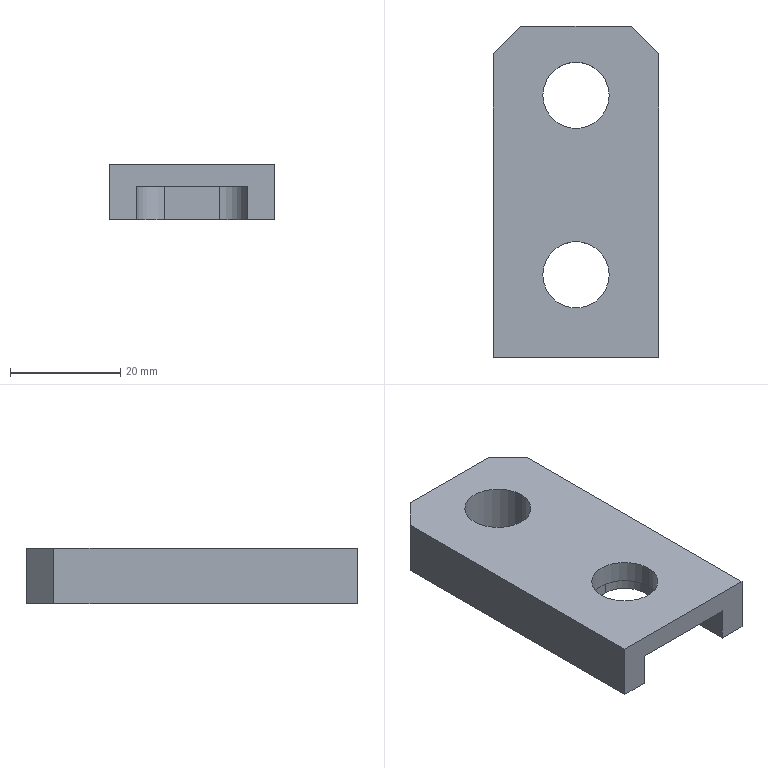Part | STEP file | Polisher connecting part | 1 solid | 18 faces | box 30 x 60 x 10 mm | volume 13231 mm3 | plane 12 | cylinder 6 | commonest cylinder face diameters 12 x4 10 x2
STEP:
#1=CARTESIAN_POINT('',(0.,0.,0.));
#2=DIRECTION('',(0.,0.,1.));
#3=DIRECTION('',(1.,0.,0.));
#4=AXIS2_PLACEMENT_3D('',#1,#2,#3);
#5=CARTESIAN_POINT('',(-6.,47.5,10.));
#6=VERTEX_POINT('',#5);
#7=CARTESIAN_POINT('',(-6.,47.5,0.));
#8=VERTEX_POINT('',#7);
#9=CARTESIAN_POINT('',(-6.,47.5,0.));
#10=DIRECTION('',(0.,0.,-1.));
#11=VECTOR('',#10,1.);
#12=LINE('',#9,#11);
#13=CARTESIAN_POINT('',(0.,47.5,0.));
#14=DIRECTION('',(0.,0.,-1.));
#15=DIRECTION('',(-1.,0.,0.));
#16=AXIS2_PLACEMENT_3D('',#13,#14,#15);
#17=CYLINDRICAL_SURFACE('',#16,6.);
#18=CARTESIAN_POINT('',(6.283,0.));
#19=DIRECTION('',(0.,1.));
#20=VECTOR('',#19,1.);
#21=LINE('',#18,#20);
#22=(GEOMETRIC_REPRESENTATION_CONTEXT(2)PARAMETRIC_REPRESENTATION_CONTEXT()REPRESENTATION_CONTEXT('',''));
#23=DEFINITIONAL_REPRESENTATION('',(#21),#22);
#24=PCURVE('',#17,#23);
#25=CARTESIAN_POINT('',(0.,47.5,0.));
#26=DIRECTION('',(0.,0.,-1.));
#27=DIRECTION('',(-1.,0.,0.));
#28=AXIS2_PLACEMENT_3D('',#25,#26,#27);
#29=CYLINDRICAL_SURFACE('',#28,6.);
#30=CARTESIAN_POINT('',(0.,0.));
#31=DIRECTION('',(0.,1.));
#32=VECTOR('',#31,1.);
#33=LINE('',#30,#32);
#34=(GEOMETRIC_REPRESENTATION_CONTEXT(2)PARAMETRIC_REPRESENTATION_CONTEXT()REPRESENTATION_CONTEXT('',''));
#35=DEFINITIONAL_REPRESENTATION('',(#33),#34);
#36=PCURVE('',#29,#35);
#37=SURFACE_CURVE('',#12,(#24,#36),.PCURVE_S1.);
#38=EDGE_CURVE('',#6,#8,#37,.T.);
#39=ORIENTED_EDGE('',*,*,#38,.T.);
#40=CARTESIAN_POINT('',(6.,47.5,0.));
#41=VERTEX_POINT('',#40);
#42=CARTESIAN_POINT('',(0.,47.5,0.));
#43=DIRECTION('',(0.,0.,-1.));
#44=DIRECTION('',(-1.,0.,0.));
#45=AXIS2_PLACEMENT_3D('',#42,#43,#44);
#46=CIRCLE('',#45,6.);
#47=CARTESIAN_POINT('',(0.,0.));
#48=DIRECTION('',(1.,0.));
#49=VECTOR('',#48,1.);
#50=LINE('',#47,#49);
#51=(GEOMETRIC_REPRESENTATION_CONTEXT(2)PARAMETRIC_REPRESENTATION_CONTEXT()REPRESENTATION_CONTEXT('',''));
#52=DEFINITIONAL_REPRESENTATION('',(#50),#51);
#53=PCURVE('',#17,#52);
#54=CARTESIAN_POINT('',(0.,0.,0.));
#55=DIRECTION('',(0.,0.,1.));
#56=DIRECTION('',(1.,0.,0.));
#57=AXIS2_PLACEMENT_3D('',#54,#55,#56);
#58=PLANE('',#57);
#59=CARTESIAN_POINT('',(-6.,47.5));
#60=CARTESIAN_POINT('',(-6.,57.892));
#61=CARTESIAN_POINT('',(3.,52.696));
#62=CARTESIAN_POINT('',(12.,47.5));
#63=CARTESIAN_POINT('',(3.,42.304));
#64=CARTESIAN_POINT('',(-6.,37.108));
#65=CARTESIAN_POINT('',(-6.,47.5));
#66=(BOUNDED_CURVE()B_SPLINE_CURVE(2,(#59,#60,#61,#62,#63,#64,#65),.UNSPECIFIED.,.T.,.F.)B_SPLINE_CURVE_WITH_KNOTS((1,2,2,2,2,1),(-2.094,0.,2.094,4.189,6.283,8.378),.UNSPECIFIED.)CURVE()GEOMETRIC_REPRESENTATION_ITEM()RATIONAL_B_SPLINE_CURVE((1.,0.5,1.,0.5,1.,0.5,1.))REPRESENTATION_ITEM(''));
#67=(GEOMETRIC_REPRESENTATION_CONTEXT(2)PARAMETRIC_REPRESENTATION_CONTEXT()REPRESENTATION_CONTEXT('',''));
#68=DEFINITIONAL_REPRESENTATION('',(#66),#67);
#69=PCURVE('',#58,#68);
#70=SURFACE_CURVE('',#46,(#53,#69),.PCURVE_S1.);
#71=EDGE_CURVE('',#41,#8,#70,.T.);
#72=ORIENTED_EDGE('',*,*,#71,.F.);
#73=CARTESIAN_POINT('',(6.,47.5,10.));
#74=VERTEX_POINT('',#73);
#75=CARTESIAN_POINT('',(6.,47.5,0.));
#76=DIRECTION('',(0.,0.,-1.));
#77=VECTOR('',#76,1.);
#78=LINE('',#75,#77);
#79=CARTESIAN_POINT('',(3.142,0.));
#80=DIRECTION('',(0.,1.));
#81=VECTOR('',#80,1.);
#82=LINE('',#79,#81);
#83=(GEOMETRIC_REPRESENTATION_CONTEXT(2)PARAMETRIC_REPRESENTATION_CONTEXT()REPRESENTATION_CONTEXT('',''));
#84=DEFINITIONAL_REPRESENTATION('',(#82),#83);
#85=PCURVE('',#17,#84);
#86=CARTESIAN_POINT('',(3.142,0.));
#87=DIRECTION('',(0.,1.));
#88=VECTOR('',#87,1.);
#89=LINE('',#86,#88);
#90=(GEOMETRIC_REPRESENTATION_CONTEXT(2)PARAMETRIC_REPRESENTATION_CONTEXT()REPRESENTATION_CONTEXT('',''));
#91=DEFINITIONAL_REPRESENTATION('',(#89),#90);
#92=PCURVE('',#29,#91);
#93=SURFACE_CURVE('',#78,(#85,#92),.PCURVE_S1.);
#94=EDGE_CURVE('',#74,#41,#93,.T.);
#95=ORIENTED_EDGE('',*,*,#94,.F.);
#96=CARTESIAN_POINT('',(0.,47.5,10.));
#97=DIRECTION('',(0.,0.,-1.));
#98=DIRECTION('',(-1.,0.,0.));
#99=AXIS2_PLACEMENT_3D('',#96,#97,#98);
#100=CIRCLE('',#99,6.);
#101=CARTESIAN_POINT('',(0.,-10.));
#102=DIRECTION('',(1.,0.));
#103=VECTOR('',#102,1.);
#104=LINE('',#101,#103);
#105=(GEOMETRIC_REPRESENTATION_CONTEXT(2)PARAMETRIC_REPRESENTATION_CONTEXT()REPRESENTATION_CONTEXT('',''));
#106=DEFINITIONAL_REPRESENTATION('',(#104),#105);
#107=PCURVE('',#17,#106);
#108=CARTESIAN_POINT('',(0.,0.,10.));
#109=DIRECTION('',(0.,0.,1.));
#110=DIRECTION('',(1.,0.,0.));
#111=AXIS2_PLACEMENT_3D('',#108,#109,#110);
#112=PLANE('',#111);
#113=CARTESIAN_POINT('',(-6.,47.5));
#114=CARTESIAN_POINT('',(-6.,57.892));
#115=CARTESIAN_POINT('',(3.,52.696));
#116=CARTESIAN_POINT('',(12.,47.5));
#117=CARTESIAN_POINT('',(3.,42.304));
#118=CARTESIAN_POINT('',(-6.,37.108));
#119=CARTESIAN_POINT('',(-6.,47.5));
#120=(BOUNDED_CURVE()B_SPLINE_CURVE(2,(#113,#114,#115,#116,#117,#118,#119),.UNSPECIFIED.,.T.,.F.)B_SPLINE_CURVE_WITH_KNOTS((1,2,2,2,2,1),(-2.094,0.,2.094,4.189,6.283,8.378),.UNSPECIFIED.)CURVE()GEOMETRIC_REPRESENTATION_ITEM()RATIONAL_B_SPLINE_CURVE((1.,0.5,1.,0.5,1.,0.5,1.))REPRESENTATION_ITEM(''));
#121=(GEOMETRIC_REPRESENTATION_CONTEXT(2)PARAMETRIC_REPRESENTATION_CONTEXT()REPRESENTATION_CONTEXT('',''));
#122=DEFINITIONAL_REPRESENTATION('',(#120),#121);
#123=PCURVE('',#112,#122);
#124=SURFACE_CURVE('',#100,(#107,#123),.PCURVE_S1.);
#125=EDGE_CURVE('',#74,#6,#124,.T.);
#126=ORIENTED_EDGE('',*,*,#125,.T.);
#127=EDGE_LOOP('',(#39,#72,#95,#126));
#128=FACE_BOUND('',#127,.F.);
#129=ADVANCED_FACE('',(#128),#17,.F.);
#130=CARTESIAN_POINT('',(-6.,15.,10.));
#131=VERTEX_POINT('',#130);
#132=CARTESIAN_POINT('',(-6.,15.,6.));
#133=VERTEX_POINT('',#132);
#134=CARTESIAN_POINT('',(-6.,15.,6.));
#135=DIRECTION('',(0.,0.,-1.));
#136=VECTOR('',#135,1.);
#137=LINE('',#134,#136);
#138=CARTESIAN_POINT('',(0.,15.,6.));
#139=DIRECTION('',(0.,0.,-1.));
#140=DIRECTION('',(-1.,0.,0.));
#141=AXIS2_PLACEMENT_3D('',#138,#139,#140);
#142=CYLINDRICAL_SURFACE('',#141,6.);
#143=CARTESIAN_POINT('',(6.283,0.));
#144=DIRECTION('',(0.,1.));
#145=VECTOR('',#144,1.);
#146=LINE('',#143,#145);
#147=(GEOMETRIC_REPRESENTATION_CONTEXT(2)PARAMETRIC_REPRESENTATION_CONTEXT()REPRESENTATION_CONTEXT('',''));
#148=DEFINITIONAL_REPRESENTATION('',(#146),#147);
#149=PCURVE('',#142,#148);
#150=CARTESIAN_POINT('',(0.,15.,6.));
#151=DIRECTION('',(0.,0.,-1.));
#152=DIRECTION('',(-1.,0.,0.));
#153=AXIS2_PLACEMENT_3D('',#150,#151,#152);
#154=CYLINDRICAL_SURFACE('',#153,6.);
#155=CARTESIAN_POINT('',(0.,0.));
#156=DIRECTION('',(0.,1.));
#157=VECTOR('',#156,1.);
#158=LINE('',#155,#157);
#159=(GEOMETRIC_REPRESENTATION_CONTEXT(2)PARAMETRIC_REPRESENTATION_CONTEXT()REPRESENTATION_CONTEXT('',''));
#160=DEFINITIONAL_REPRESENTATION('',(#158),#159);
#161=PCURVE('',#154,#160);
#162=SURFACE_CURVE('',#137,(#149,#161),.PCURVE_S1.);
#163=EDGE_CURVE('',#131,#133,#162,.T.);
#164=ORIENTED_EDGE('',*,*,#163,.T.);
#165=CARTESIAN_POINT('',(6.,15.,6.));
#166=VERTEX_POINT('',#165);
#167=CARTESIAN_POINT('',(0.,15.,6.));
#168=DIRECTION('',(0.,0.,-1.));
#169=DIRECTION('',(-1.,0.,0.));
#170=AXIS2_PLACEMENT_3D('',#167,#168,#169);
#171=CIRCLE('',#170,6.);
#172=CARTESIAN_POINT('',(0.,0.));
#173=DIRECTION('',(1.,0.));
#174=VECTOR('',#173,1.);
#175=LINE('',#172,#174);
#176=(GEOMETRIC_REPRESENTATION_CONTEXT(2)PARAMETRIC_REPRESENTATION_CONTEXT()REPRESENTATION_CONTEXT('',''));
#177=DEFINITIONAL_REPRESENTATION('',(#175),#176);
#178=PCURVE('',#142,#177);
#179=CARTESIAN_POINT('',(0.,0.,6.));
#180=DIRECTION('',(0.,0.,1.));
#181=DIRECTION('',(1.,0.,0.));
#182=AXIS2_PLACEMENT_3D('',#179,#180,#181);
#183=PLANE('',#182);
#184=CARTESIAN_POINT('',(-6.,15.));
#185=CARTESIAN_POINT('',(-6.,25.392));
#186=CARTESIAN_POINT('',(3.,20.196));
#187=CARTESIAN_POINT('',(12.,15.));
#188=CARTESIAN_POINT('',(3.,9.804));
#189=CARTESIAN_POINT('',(-6.,4.608));
#190=CARTESIAN_POINT('',(-6.,15.));
#191=(BOUNDED_CURVE()B_SPLINE_CURVE(2,(#184,#185,#186,#187,#188,#189,#190),.UNSPECIFIED.,.T.,.F.)B_SPLINE_CURVE_WITH_KNOTS((1,2,2,2,2,1),(-2.094,0.,2.094,4.189,6.283,8.378),.UNSPECIFIED.)CURVE()GEOMETRIC_REPRESENTATION_ITEM()RATIONAL_B_SPLINE_CURVE((1.,0.5,1.,0.5,1.,0.5,1.))REPRESENTATION_ITEM(''));
#192=(GEOMETRIC_REPRESENTATION_CONTEXT(2)PARAMETRIC_REPRESENTATION_CONTEXT()REPRESENTATION_CONTEXT('',''));
#193=DEFINITIONAL_REPRESENTATION('',(#191),#192);
#194=PCURVE('',#183,#193);
#195=SURFACE_CURVE('',#171,(#178,#194),.PCURVE_S1.);
#196=EDGE_CURVE('',#166,#133,#195,.T.);
#197=ORIENTED_EDGE('',*,*,#196,.F.);
#198=CARTESIAN_POINT('',(6.,15.,10.));
#199=VERTEX_POINT('',#198);
#200=CARTESIAN_POINT('',(6.,15.,6.));
#201=DIRECTION('',(0.,0.,-1.));
#202=VECTOR('',#201,1.);
#203=LINE('',#200,#202);
#204=CARTESIAN_POINT('',(3.142,0.));
#205=DIRECTION('',(0.,1.));
#206=VECTOR('',#205,1.);
#207=LINE('',#204,#206);
#208=(GEOMETRIC_REPRESENTATION_CONTEXT(2)PARAMETRIC_REPRESENTATION_CONTEXT()REPRESENTATION_CONTEXT('',''));
#209=DEFINITIONAL_REPRESENTATION('',(#207),#208);
#210=PCURVE('',#142,#209);
#211=CARTESIAN_POINT('',(3.142,0.));
#212=DIRECTION('',(0.,1.));
#213=VECTOR('',#212,1.);
#214=LINE('',#211,#213);
#215=(GEOMETRIC_REPRESENTATION_CONTEXT(2)PARAMETRIC_REPRESENTATION_CONTEXT()REPRESENTATION_CONTEXT('',''));
#216=DEFINITIONAL_REPRESENTATION('',(#214),#215);
#217=PCURVE('',#154,#216);
#218=SURFACE_CURVE('',#203,(#210,#217),.PCURVE_S1.);
#219=EDGE_CURVE('',#199,#166,#218,.T.);
#220=ORIENTED_EDGE('',*,*,#219,.F.);
#221=CARTESIAN_POINT('',(0.,15.,10.));
#222=DIRECTION('',(0.,0.,1.));
#223=DIRECTION('',(1.,0.,0.));
#224=AXIS2_PLACEMENT_3D('',#221,#222,#223);
#225=CIRCLE('',#224,6.);
#226=CARTESIAN_POINT('',(9.425,-4.));
#227=DIRECTION('',(-1.,0.));
#228=VECTOR('',#227,1.);
#229=LINE('',#226,#228);
#230=(GEOMETRIC_REPRESENTATION_CONTEXT(2)PARAMETRIC_REPRESENTATION_CONTEXT()REPRESENTATION_CONTEXT('',''));
#231=DEFINITIONAL_REPRESENTATION('',(#229),#230);
#232=PCURVE('',#142,#231);
#233=CARTESIAN_POINT('',(0.,15.));
#234=DIRECTION('',(1.,0.));
#235=AXIS2_PLACEMENT_2D('',#233,#234);
#236=CIRCLE('',#235,6.);
#237=(GEOMETRIC_REPRESENTATION_CONTEXT(2)PARAMETRIC_REPRESENTATION_CONTEXT()REPRESENTATION_CONTEXT('',''));
#238=DEFINITIONAL_REPRESENTATION('',(#236),#237);
#239=PCURVE('',#112,#238);
#240=SURFACE_CURVE('',#225,(#232,#239),.PCURVE_S1.);
#241=EDGE_CURVE('',#131,#199,#240,.T.);
#242=ORIENTED_EDGE('',*,*,#241,.F.);
#243=EDGE_LOOP('',(#164,#197,#220,#242));
#244=FACE_BOUND('',#243,.F.);
#245=ADVANCED_FACE('',(#244),#142,.F.);
#246=CARTESIAN_POINT('',(0.,47.5,0.));
#247=DIRECTION('',(0.,0.,-1.));
#248=DIRECTION('',(-1.,0.,0.));
#249=AXIS2_PLACEMENT_3D('',#246,#247,#248);
#250=CIRCLE('',#249,6.);
#251=CARTESIAN_POINT('',(-6.,47.5));
#252=CARTESIAN_POINT('',(-6.,57.892));
#253=CARTESIAN_POINT('',(3.,52.696));
#254=CARTESIAN_POINT('',(12.,47.5));
#255=CARTESIAN_POINT('',(3.,42.304));
#256=CARTESIAN_POINT('',(-6.,37.108));
#257=CARTESIAN_POINT('',(-6.,47.5));
#258=(BOUNDED_CURVE()B_SPLINE_CURVE(2,(#251,#252,#253,#254,#255,#256,#257),.UNSPECIFIED.,.T.,.F.)B_SPLINE_CURVE_WITH_KNOTS((1,2,2,2,2,1),(-2.094,0.,2.094,4.189,6.283,8.378),.UNSPECIFIED.)CURVE()GEOMETRIC_REPRESENTATION_ITEM()RATIONAL_B_SPLINE_CURVE((1.,0.5,1.,0.5,1.,0.5,1.))REPRESENTATION_ITEM(''));
#259=(GEOMETRIC_REPRESENTATION_CONTEXT(2)PARAMETRIC_REPRESENTATION_CONTEXT()REPRESENTATION_CONTEXT('',''));
#260=DEFINITIONAL_REPRESENTATION('',(#258),#259);
#261=PCURVE('',#58,#260);
#262=CARTESIAN_POINT('',(0.,0.));
#263=DIRECTION('',(1.,0.));
#264=VECTOR('',#263,1.);
#265=LINE('',#262,#264);
#266=(GEOMETRIC_REPRESENTATION_CONTEXT(2)PARAMETRIC_REPRESENTATION_CONTEXT()REPRESENTATION_CONTEXT('',''));
#267=DEFINITIONAL_REPRESENTATION('',(#265),#266);
#268=PCURVE('',#29,#267);
#269=SURFACE_CURVE('',#250,(#261,#268),.PCURVE_S1.);
#270=EDGE_CURVE('',#8,#41,#269,.T.);
#271=ORIENTED_EDGE('',*,*,#270,.F.);
#272=ORIENTED_EDGE('',*,*,#71,.F.);
#273=EDGE_LOOP('',(#271,#272));
#274=FACE_BOUND('',#273,.T.);
#275=CARTESIAN_POINT('',(10.,60.,0.));
#276=VERTEX_POINT('',#275);
#277=CARTESIAN_POINT('',(-10.,60.,0.));
#278=VERTEX_POINT('',#277);
#279=CARTESIAN_POINT('',(15.,60.,0.));
#280=DIRECTION('',(-1.,0.,0.));
#281=VECTOR('',#280,1.);
#282=LINE('',#279,#281);
#283=CARTESIAN_POINT('',(15.,60.));
#284=DIRECTION('',(-1.,0.));
#285=VECTOR('',#284,1.);
#286=LINE('',#283,#285);
#287=(GEOMETRIC_REPRESENTATION_CONTEXT(2)PARAMETRIC_REPRESENTATION_CONTEXT()REPRESENTATION_CONTEXT('',''));
#288=DEFINITIONAL_REPRESENTATION('',(#286),#287);
#289=PCURVE('',#58,#288);
#290=CARTESIAN_POINT('',(15.,60.,43.541));
#291=DIRECTION('',(0.,-1.,0.));
#292=DIRECTION('',(1.,0.,0.));
#293=AXIS2_PLACEMENT_3D('',#290,#291,#292);
#294=PLANE('',#293);
#295=CARTESIAN_POINT('',(0.,-43.541));
#296=DIRECTION('',(-1.,0.));
#297=VECTOR('',#296,1.);
#298=LINE('',#295,#297);
#299=(GEOMETRIC_REPRESENTATION_CONTEXT(2)PARAMETRIC_REPRESENTATION_CONTEXT()REPRESENTATION_CONTEXT('',''));
#300=DEFINITIONAL_REPRESENTATION('',(#298),#299);
#301=PCURVE('',#294,#300);
#302=SURFACE_CURVE('',#282,(#289,#301),.PCURVE_S1.);
#303=EDGE_CURVE('',#276,#278,#302,.T.);
#304=ORIENTED_EDGE('',*,*,#303,.F.);
#305=CARTESIAN_POINT('',(15.,55.,0.));
#306=VERTEX_POINT('',#305);
#307=CARTESIAN_POINT('',(10.,60.,0.));
#308=DIRECTION('',(0.7071,-0.7071,0.));
#309=VECTOR('',#308,1.);
#310=LINE('',#307,#309);
#311=CARTESIAN_POINT('',(10.,60.));
#312=DIRECTION('',(0.7071,-0.7071));
#313=VECTOR('',#312,1.);
#314=LINE('',#311,#313);
#315=(GEOMETRIC_REPRESENTATION_CONTEXT(2)PARAMETRIC_REPRESENTATION_CONTEXT()REPRESENTATION_CONTEXT('',''));
#316=DEFINITIONAL_REPRESENTATION('',(#314),#315);
#317=PCURVE('',#58,#316);
#318=CARTESIAN_POINT('',(10.,60.,43.541));
#319=DIRECTION('',(-0.7071,-0.7071,0.));
#320=DIRECTION('',(0.,0.,-1.));
#321=AXIS2_PLACEMENT_3D('',#318,#319,#320);
#322=PLANE('',#321);
#323=CARTESIAN_POINT('',(43.541,0.));
#324=DIRECTION('',(0.,1.));
#325=VECTOR('',#324,1.);
#326=LINE('',#323,#325);
#327=(GEOMETRIC_REPRESENTATION_CONTEXT(2)PARAMETRIC_REPRESENTATION_CONTEXT()REPRESENTATION_CONTEXT('',''));
#328=DEFINITIONAL_REPRESENTATION('',(#326),#327);
#329=PCURVE('',#322,#328);
#330=SURFACE_CURVE('',#310,(#317,#329),.PCURVE_S1.);
#331=EDGE_CURVE('',#276,#306,#330,.T.);
#332=ORIENTED_EDGE('',*,*,#331,.T.);
#333=CARTESIAN_POINT('',(15.,0.,0.));
#334=VERTEX_POINT('',#333);
#335=CARTESIAN_POINT('',(15.,0.,0.));
#336=DIRECTION('',(0.,1.,0.));
#337=VECTOR('',#336,1.);
#338=LINE('',#335,#337);
#339=CARTESIAN_POINT('',(15.,0.));
#340=DIRECTION('',(0.,1.));
#341=VECTOR('',#340,1.);
#342=LINE('',#339,#341);
#343=(GEOMETRIC_REPRESENTATION_CONTEXT(2)PARAMETRIC_REPRESENTATION_CONTEXT()REPRESENTATION_CONTEXT('',''));
#344=DEFINITIONAL_REPRESENTATION('',(#342),#343);
#345=PCURVE('',#58,#344);
#346=CARTESIAN_POINT('',(15.,0.,10.));
#347=DIRECTION('',(-1.,0.,0.));
#348=DIRECTION('',(0.,0.,1.));
#349=AXIS2_PLACEMENT_3D('',#346,#347,#348);
#350=PLANE('',#349);
#351=CARTESIAN_POINT('',(-10.,0.));
#352=DIRECTION('',(0.,1.));
#353=VECTOR('',#352,1.);
#354=LINE('',#351,#353);
#355=(GEOMETRIC_REPRESENTATION_CONTEXT(2)PARAMETRIC_REPRESENTATION_CONTEXT()REPRESENTATION_CONTEXT('',''));
#356=DEFINITIONAL_REPRESENTATION('',(#354),#355);
#357=PCURVE('',#350,#356);
#358=SURFACE_CURVE('',#338,(#345,#357),.PCURVE_S1.);
#359=EDGE_CURVE('',#334,#306,#358,.T.);
#360=ORIENTED_EDGE('',*,*,#359,.F.);
#361=CARTESIAN_POINT('',(10.,0.,0.));
#362=VERTEX_POINT('',#361);
#363=CARTESIAN_POINT('',(0.,0.,0.));
#364=DIRECTION('',(-1.,0.,0.));
#365=VECTOR('',#364,1.);
#366=LINE('',#363,#365);
#367=CARTESIAN_POINT('',(0.,0.));
#368=DIRECTION('',(-1.,0.));
#369=VECTOR('',#368,1.);
#370=LINE('',#367,#369);
#371=(GEOMETRIC_REPRESENTATION_CONTEXT(2)PARAMETRIC_REPRESENTATION_CONTEXT()REPRESENTATION_CONTEXT('',''));
#372=DEFINITIONAL_REPRESENTATION('',(#370),#371);
#373=PCURVE('',#58,#372);
#374=CARTESIAN_POINT('',(15.,0.,10.));
#375=DIRECTION('',(0.,1.,0.));
#376=DIRECTION('',(0.,0.,1.));
#377=AXIS2_PLACEMENT_3D('',#374,#375,#376);
#378=PLANE('',#377);
#379=CARTESIAN_POINT('',(-10.,-15.));
#380=DIRECTION('',(0.,-1.));
#381=VECTOR('',#380,1.);
#382=LINE('',#379,#381);
#383=(GEOMETRIC_REPRESENTATION_CONTEXT(2)PARAMETRIC_REPRESENTATION_CONTEXT()REPRESENTATION_CONTEXT('',''));
#384=DEFINITIONAL_REPRESENTATION('',(#382),#383);
#385=PCURVE('',#378,#384);
#386=SURFACE_CURVE('',#366,(#373,#385),.PCURVE_S1.);
#387=EDGE_CURVE('',#334,#362,#386,.T.);
#388=ORIENTED_EDGE('',*,*,#387,.T.);
#389=CARTESIAN_POINT('',(10.,20.,0.));
#390=VERTEX_POINT('',#389);
#391=CARTESIAN_POINT('',(10.,-25.,0.));
#392=DIRECTION('',(0.,1.,0.));
#393=VECTOR('',#392,1.);
#394=LINE('',#391,#393);
#395=CARTESIAN_POINT('',(10.,-25.));
#396=DIRECTION('',(0.,1.));
#397=VECTOR('',#396,1.);
#398=LINE('',#395,#397);
#399=(GEOMETRIC_REPRESENTATION_CONTEXT(2)PARAMETRIC_REPRESENTATION_CONTEXT()REPRESENTATION_CONTEXT('',''));
#400=DEFINITIONAL_REPRESENTATION('',(#398),#399);
#401=PCURVE('',#58,#400);
#402=CARTESIAN_POINT('',(10.,-25.,6.));
#403=DIRECTION('',(-1.,0.,0.));
#404=DIRECTION('',(0.,0.,1.));
#405=AXIS2_PLACEMENT_3D('',#402,#403,#404);
#406=PLANE('',#405);
#407=CARTESIAN_POINT('',(-6.,0.));
#408=DIRECTION('',(0.,1.));
#409=VECTOR('',#408,1.);
#410=LINE('',#407,#409);
#411=(GEOMETRIC_REPRESENTATION_CONTEXT(2)PARAMETRIC_REPRESENTATION_CONTEXT()REPRESENTATION_CONTEXT('',''));
#412=DEFINITIONAL_REPRESENTATION('',(#410),#411);
#413=PCURVE('',#406,#412);
#414=SURFACE_CURVE('',#394,(#401,#413),.PCURVE_S1.);
#415=EDGE_CURVE('',#362,#390,#414,.T.);
#416=ORIENTED_EDGE('',*,*,#415,.T.);
#417=CARTESIAN_POINT('',(5.,25.,0.));
#418=VERTEX_POINT('',#417);
#419=CARTESIAN_POINT('',(5.,20.,0.));
#420=DIRECTION('',(0.,0.,1.));
#421=DIRECTION('',(1.,0.,0.));
#422=AXIS2_PLACEMENT_3D('',#419,#420,#421);
#423=CIRCLE('',#422,5.);
#424=CARTESIAN_POINT('',(5.,20.));
#425=DIRECTION('',(1.,0.));
#426=AXIS2_PLACEMENT_2D('',#424,#425);
#427=CIRCLE('',#426,5.);
#428=(GEOMETRIC_REPRESENTATION_CONTEXT(2)PARAMETRIC_REPRESENTATION_CONTEXT()REPRESENTATION_CONTEXT('',''));
#429=DEFINITIONAL_REPRESENTATION('',(#427),#428);
#430=PCURVE('',#58,#429);
#431=CARTESIAN_POINT('',(5.,20.,6.));
#432=DIRECTION('',(0.,0.,1.));
#433=DIRECTION('',(1.,0.,0.));
#434=AXIS2_PLACEMENT_3D('',#431,#432,#433);
#435=CYLINDRICAL_SURFACE('',#434,5.);
#436=CARTESIAN_POINT('',(0.,-6.));
#437=DIRECTION('',(1.,0.));
#438=VECTOR('',#437,1.);
#439=LINE('',#436,#438);
#440=(GEOMETRIC_REPRESENTATION_CONTEXT(2)PARAMETRIC_REPRESENTATION_CONTEXT()REPRESENTATION_CONTEXT('',''));
#441=DEFINITIONAL_REPRESENTATION('',(#439),#440);
#442=PCURVE('',#435,#441);
#443=SURFACE_CURVE('',#423,(#430,#442),.PCURVE_S1.);
#444=EDGE_CURVE('',#390,#418,#443,.T.);
#445=ORIENTED_EDGE('',*,*,#444,.T.);
#446=CARTESIAN_POINT('',(-5.,25.,0.));
#447=VERTEX_POINT('',#446);
#448=CARTESIAN_POINT('',(10.,25.,0.));
#449=DIRECTION('',(-1.,0.,0.));
#450=VECTOR('',#449,1.);
#451=LINE('',#448,#450);
#452=CARTESIAN_POINT('',(10.,25.));
#453=DIRECTION('',(-1.,0.));
#454=VECTOR('',#453,1.);
#455=LINE('',#452,#454);
#456=(GEOMETRIC_REPRESENTATION_CONTEXT(2)PARAMETRIC_REPRESENTATION_CONTEXT()REPRESENTATION_CONTEXT('',''));
#457=DEFINITIONAL_REPRESENTATION('',(#455),#456);
#458=PCURVE('',#58,#457);
#459=CARTESIAN_POINT('',(10.,25.,6.));
#460=DIRECTION('',(0.,-1.,0.));
#461=DIRECTION('',(0.,0.,-1.));
#462=AXIS2_PLACEMENT_3D('',#459,#460,#461);
#463=PLANE('',#462);
#464=CARTESIAN_POINT('',(6.,0.));
#465=DIRECTION('',(0.,-1.));
#466=VECTOR('',#465,1.);
#467=LINE('',#464,#466);
#468=(GEOMETRIC_REPRESENTATION_CONTEXT(2)PARAMETRIC_REPRESENTATION_CONTEXT()REPRESENTATION_CONTEXT('',''));
#469=DEFINITIONAL_REPRESENTATION('',(#467),#468);
#470=PCURVE('',#463,#469);
#471=SURFACE_CURVE('',#451,(#458,#470),.PCURVE_S1.);
#472=EDGE_CURVE('',#418,#447,#471,.T.);
#473=ORIENTED_EDGE('',*,*,#472,.T.);
#474=CARTESIAN_POINT('',(-10.,20.,0.));
#475=VERTEX_POINT('',#474);
#476=CARTESIAN_POINT('',(-5.,20.,0.));
#477=DIRECTION('',(0.,0.,1.));
#478=DIRECTION('',(1.,0.,0.));
#479=AXIS2_PLACEMENT_3D('',#476,#477,#478);
#480=CIRCLE('',#479,5.);
#481=CARTESIAN_POINT('',(-5.,20.));
#482=DIRECTION('',(1.,0.));
#483=AXIS2_PLACEMENT_2D('',#481,#482);
#484=CIRCLE('',#483,5.);
#485=(GEOMETRIC_REPRESENTATION_CONTEXT(2)PARAMETRIC_REPRESENTATION_CONTEXT()REPRESENTATION_CONTEXT('',''));
#486=DEFINITIONAL_REPRESENTATION('',(#484),#485);
#487=PCURVE('',#58,#486);
#488=CARTESIAN_POINT('',(-5.,20.,6.));
#489=DIRECTION('',(0.,0.,1.));
#490=DIRECTION('',(1.,0.,0.));
#491=AXIS2_PLACEMENT_3D('',#488,#489,#490);
#492=CYLINDRICAL_SURFACE('',#491,5.);
#493=CARTESIAN_POINT('',(0.,-6.));
#494=DIRECTION('',(1.,0.));
#495=VECTOR('',#494,1.);
#496=LINE('',#493,#495);
#497=(GEOMETRIC_REPRESENTATION_CONTEXT(2)PARAMETRIC_REPRESENTATION_CONTEXT()REPRESENTATION_CONTEXT('',''));
#498=DEFINITIONAL_REPRESENTATION('',(#496),#497);
#499=PCURVE('',#492,#498);
#500=SURFACE_CURVE('',#480,(#487,#499),.PCURVE_S1.);
#501=EDGE_CURVE('',#447,#475,#500,.T.);
#502=ORIENTED_EDGE('',*,*,#501,.T.);
#503=CARTESIAN_POINT('',(-10.,0.,0.));
#504=VERTEX_POINT('',#503);
#505=CARTESIAN_POINT('',(-10.,-25.,0.));
#506=DIRECTION('',(0.,-1.,0.));
#507=VECTOR('',#506,1.);
#508=LINE('',#505,#507);
#509=CARTESIAN_POINT('',(-10.,-25.));
#510=DIRECTION('',(0.,-1.));
#511=VECTOR('',#510,1.);
#512=LINE('',#509,#511);
#513=(GEOMETRIC_REPRESENTATION_CONTEXT(2)PARAMETRIC_REPRESENTATION_CONTEXT()REPRESENTATION_CONTEXT('',''));
#514=DEFINITIONAL_REPRESENTATION('',(#512),#513);
#515=PCURVE('',#58,#514);
#516=CARTESIAN_POINT('',(-10.,-25.,6.));
#517=DIRECTION('',(1.,0.,0.));
#518=DIRECTION('',(0.,0.,-1.));
#519=AXIS2_PLACEMENT_3D('',#516,#517,#518);
#520=PLANE('',#519);
#521=CARTESIAN_POINT('',(6.,0.));
#522=DIRECTION('',(0.,-1.));
#523=VECTOR('',#522,1.);
#524=LINE('',#521,#523);
#525=(GEOMETRIC_REPRESENTATION_CONTEXT(2)PARAMETRIC_REPRESENTATION_CONTEXT()REPRESENTATION_CONTEXT('',''));
#526=DEFINITIONAL_REPRESENTATION('',(#524),#525);
#527=PCURVE('',#520,#526);
#528=SURFACE_CURVE('',#508,(#515,#527),.PCURVE_S1.);
#529=EDGE_CURVE('',#475,#504,#528,.T.);
#530=ORIENTED_EDGE('',*,*,#529,.T.);
#531=CARTESIAN_POINT('',(-15.,0.,0.));
#532=VERTEX_POINT('',#531);
#533=CARTESIAN_POINT('',(0.,0.,0.));
#534=DIRECTION('',(-1.,0.,0.));
#535=VECTOR('',#534,1.);
#536=LINE('',#533,#535);
#537=CARTESIAN_POINT('',(0.,0.));
#538=DIRECTION('',(-1.,0.));
#539=VECTOR('',#538,1.);
#540=LINE('',#537,#539);
#541=(GEOMETRIC_REPRESENTATION_CONTEXT(2)PARAMETRIC_REPRESENTATION_CONTEXT()REPRESENTATION_CONTEXT('',''));
#542=DEFINITIONAL_REPRESENTATION('',(#540),#541);
#543=PCURVE('',#58,#542);
#544=CARTESIAN_POINT('',(-10.,-15.));
#545=DIRECTION('',(0.,-1.));
#546=VECTOR('',#545,1.);
#547=LINE('',#544,#546);
#548=(GEOMETRIC_REPRESENTATION_CONTEXT(2)PARAMETRIC_REPRESENTATION_CONTEXT()REPRESENTATION_CONTEXT('',''));
#549=DEFINITIONAL_REPRESENTATION('',(#547),#548);
#550=PCURVE('',#378,#549);
#551=SURFACE_CURVE('',#536,(#543,#550),.PCURVE_S1.);
#552=EDGE_CURVE('',#504,#532,#551,.T.);
#553=ORIENTED_EDGE('',*,*,#552,.T.);
#554=CARTESIAN_POINT('',(-15.,55.,0.));
#555=VERTEX_POINT('',#554);
#556=CARTESIAN_POINT('',(-15.,0.,0.));
#557=DIRECTION('',(0.,-1.,0.));
#558=VECTOR('',#557,1.);
#559=LINE('',#556,#558);
#560=CARTESIAN_POINT('',(-15.,0.));
#561=DIRECTION('',(0.,-1.));
#562=VECTOR('',#561,1.);
#563=LINE('',#560,#562);
#564=(GEOMETRIC_REPRESENTATION_CONTEXT(2)PARAMETRIC_REPRESENTATION_CONTEXT()REPRESENTATION_CONTEXT('',''));
#565=DEFINITIONAL_REPRESENTATION('',(#563),#564);
#566=PCURVE('',#58,#565);
#567=CARTESIAN_POINT('',(-15.,0.,10.));
#568=DIRECTION('',(1.,0.,0.));
#569=DIRECTION('',(0.,0.,-1.));
#570=AXIS2_PLACEMENT_3D('',#567,#568,#569);
#571=PLANE('',#570);
#572=CARTESIAN_POINT('',(10.,0.));
#573=DIRECTION('',(0.,-1.));
#574=VECTOR('',#573,1.);
#575=LINE('',#572,#574);
#576=(GEOMETRIC_REPRESENTATION_CONTEXT(2)PARAMETRIC_REPRESENTATION_CONTEXT()REPRESENTATION_CONTEXT('',''));
#577=DEFINITIONAL_REPRESENTATION('',(#575),#576);
#578=PCURVE('',#571,#577);
#579=SURFACE_CURVE('',#559,(#566,#578),.PCURVE_S1.);
#580=EDGE_CURVE('',#555,#532,#579,.T.);
#581=ORIENTED_EDGE('',*,*,#580,.F.);
#582=CARTESIAN_POINT('',(-15.,55.,0.));
#583=DIRECTION('',(0.7071,0.7071,0.));
#584=VECTOR('',#583,1.);
#585=LINE('',#582,#584);
#586=CARTESIAN_POINT('',(-15.,55.));
#587=DIRECTION('',(0.7071,0.7071));
#588=VECTOR('',#587,1.);
#589=LINE('',#586,#588);
#590=(GEOMETRIC_REPRESENTATION_CONTEXT(2)PARAMETRIC_REPRESENTATION_CONTEXT()REPRESENTATION_CONTEXT('',''));
#591=DEFINITIONAL_REPRESENTATION('',(#589),#590);
#592=PCURVE('',#58,#591);
#593=CARTESIAN_POINT('',(-15.,55.,10.));
#594=DIRECTION('',(0.7071,-0.7071,0.));
#595=DIRECTION('',(0.,0.,-1.));
#596=AXIS2_PLACEMENT_3D('',#593,#594,#595);
#597=PLANE('',#596);
#598=CARTESIAN_POINT('',(10.,0.));
#599=DIRECTION('',(0.,1.));
#600=VECTOR('',#599,1.);
#601=LINE('',#598,#600);
#602=(GEOMETRIC_REPRESENTATION_CONTEXT(2)PARAMETRIC_REPRESENTATION_CONTEXT()REPRESENTATION_CONTEXT('',''));
#603=DEFINITIONAL_REPRESENTATION('',(#601),#602);
#604=PCURVE('',#597,#603);
#605=SURFACE_CURVE('',#585,(#592,#604),.PCURVE_S1.);
#606=EDGE_CURVE('',#555,#278,#605,.T.);
#607=ORIENTED_EDGE('',*,*,#606,.T.);
#608=EDGE_LOOP('',(#304,#332,#360,#388,#416,#445,#473,#502,#530,#553,#581,#607));
#609=FACE_BOUND('',#608,.T.);
#610=ADVANCED_FACE('',(#274,#609),#58,.F.);
#611=CARTESIAN_POINT('',(-10.,0.,6.));
#612=VERTEX_POINT('',#611);
#613=CARTESIAN_POINT('',(-10.,0.,10.));
#614=DIRECTION('',(0.,0.,-1.));
#615=VECTOR('',#614,1.);
#616=LINE('',#613,#615);
#617=CARTESIAN_POINT('',(0.,-25.));
#618=DIRECTION('',(-1.,0.));
#619=VECTOR('',#618,1.);
#620=LINE('',#617,#619);
#621=(GEOMETRIC_REPRESENTATION_CONTEXT(2)PARAMETRIC_REPRESENTATION_CONTEXT()REPRESENTATION_CONTEXT('',''));
#622=DEFINITIONAL_REPRESENTATION('',(#620),#621);
#623=PCURVE('',#378,#622);
#624=CARTESIAN_POINT('',(-4.,25.));
#625=DIRECTION('',(1.,0.));
#626=VECTOR('',#625,1.);
#627=LINE('',#624,#626);
#628=(GEOMETRIC_REPRESENTATION_CONTEXT(2)PARAMETRIC_REPRESENTATION_CONTEXT()REPRESENTATION_CONTEXT('',''));
#629=DEFINITIONAL_REPRESENTATION('',(#627),#628);
#630=PCURVE('',#520,#629);
#631=SURFACE_CURVE('',#616,(#623,#630),.PCURVE_S1.);
#632=EDGE_CURVE('',#612,#504,#631,.T.);
#633=ORIENTED_EDGE('',*,*,#632,.F.);
#634=CARTESIAN_POINT('',(10.,0.,6.));
#635=VERTEX_POINT('',#634);
#636=CARTESIAN_POINT('',(15.,0.,6.));
#637=DIRECTION('',(1.,0.,0.));
#638=VECTOR('',#637,1.);
#639=LINE('',#636,#638);
#640=CARTESIAN_POINT('',(-4.,0.));
#641=DIRECTION('',(0.,1.));
#642=VECTOR('',#641,1.);
#643=LINE('',#640,#642);
#644=(GEOMETRIC_REPRESENTATION_CONTEXT(2)PARAMETRIC_REPRESENTATION_CONTEXT()REPRESENTATION_CONTEXT('',''));
#645=DEFINITIONAL_REPRESENTATION('',(#643),#644);
#646=PCURVE('',#378,#645);
#647=CARTESIAN_POINT('',(15.,0.));
#648=DIRECTION('',(1.,0.));
#649=VECTOR('',#648,1.);
#650=LINE('',#647,#649);
#651=(GEOMETRIC_REPRESENTATION_CONTEXT(2)PARAMETRIC_REPRESENTATION_CONTEXT()REPRESENTATION_CONTEXT('',''));
#652=DEFINITIONAL_REPRESENTATION('',(#650),#651);
#653=PCURVE('',#183,#652);
#654=SURFACE_CURVE('',#639,(#646,#653),.PCURVE_S1.);
#655=EDGE_CURVE('',#612,#635,#654,.T.);
#656=ORIENTED_EDGE('',*,*,#655,.T.);
#657=CARTESIAN_POINT('',(10.,0.,10.));
#658=DIRECTION('',(0.,0.,1.));
#659=VECTOR('',#658,1.);
#660=LINE('',#657,#659);
#661=CARTESIAN_POINT('',(0.,-5.));
#662=DIRECTION('',(1.,0.));
#663=VECTOR('',#662,1.);
#664=LINE('',#661,#663);
#665=(GEOMETRIC_REPRESENTATION_CONTEXT(2)PARAMETRIC_REPRESENTATION_CONTEXT()REPRESENTATION_CONTEXT('',''));
#666=DEFINITIONAL_REPRESENTATION('',(#664),#665);
#667=PCURVE('',#378,#666);
#668=CARTESIAN_POINT('',(4.,25.));
#669=DIRECTION('',(1.,0.));
#670=VECTOR('',#669,1.);
#671=LINE('',#668,#670);
#672=(GEOMETRIC_REPRESENTATION_CONTEXT(2)PARAMETRIC_REPRESENTATION_CONTEXT()REPRESENTATION_CONTEXT('',''));
#673=DEFINITIONAL_REPRESENTATION('',(#671),#672);
#674=PCURVE('',#406,#673);
#675=SURFACE_CURVE('',#660,(#667,#674),.PCURVE_S1.);
#676=EDGE_CURVE('',#362,#635,#675,.T.);
#677=ORIENTED_EDGE('',*,*,#676,.F.);
#678=ORIENTED_EDGE('',*,*,#387,.F.);
#679=CARTESIAN_POINT('',(15.,0.,10.));
#680=VERTEX_POINT('',#679);
#681=CARTESIAN_POINT('',(15.,0.,10.));
#682=DIRECTION('',(0.,0.,-1.));
#683=VECTOR('',#682,1.);
#684=LINE('',#681,#683);
#685=CARTESIAN_POINT('',(0.,0.));
#686=DIRECTION('',(-1.,0.));
#687=VECTOR('',#686,1.);
#688=LINE('',#685,#687);
#689=(GEOMETRIC_REPRESENTATION_CONTEXT(2)PARAMETRIC_REPRESENTATION_CONTEXT()REPRESENTATION_CONTEXT('',''));
#690=DEFINITIONAL_REPRESENTATION('',(#688),#689);
#691=PCURVE('',#378,#690);
#692=CARTESIAN_POINT('',(0.,0.));
#693=DIRECTION('',(-1.,0.));
#694=VECTOR('',#693,1.);
#695=LINE('',#692,#694);
#696=(GEOMETRIC_REPRESENTATION_CONTEXT(2)PARAMETRIC_REPRESENTATION_CONTEXT()REPRESENTATION_CONTEXT('',''));
#697=DEFINITIONAL_REPRESENTATION('',(#695),#696);
#698=PCURVE('',#350,#697);
#699=SURFACE_CURVE('',#684,(#691,#698),.PCURVE_S1.);
#700=EDGE_CURVE('',#680,#334,#699,.T.);
#701=ORIENTED_EDGE('',*,*,#700,.F.);
#702=CARTESIAN_POINT('',(-15.,0.,10.));
#703=VERTEX_POINT('',#702);
#704=CARTESIAN_POINT('',(15.,0.,10.));
#705=DIRECTION('',(1.,0.,0.));
#706=VECTOR('',#705,1.);
#707=LINE('',#704,#706);
#708=CARTESIAN_POINT('',(0.,0.));
#709=DIRECTION('',(0.,1.));
#710=VECTOR('',#709,1.);
#711=LINE('',#708,#710);
#712=(GEOMETRIC_REPRESENTATION_CONTEXT(2)PARAMETRIC_REPRESENTATION_CONTEXT()REPRESENTATION_CONTEXT('',''));
#713=DEFINITIONAL_REPRESENTATION('',(#711),#712);
#714=PCURVE('',#378,#713);
#715=CARTESIAN_POINT('',(15.,0.));
#716=DIRECTION('',(1.,0.));
#717=VECTOR('',#716,1.);
#718=LINE('',#715,#717);
#719=(GEOMETRIC_REPRESENTATION_CONTEXT(2)PARAMETRIC_REPRESENTATION_CONTEXT()REPRESENTATION_CONTEXT('',''));
#720=DEFINITIONAL_REPRESENTATION('',(#718),#719);
#721=PCURVE('',#112,#720);
#722=SURFACE_CURVE('',#707,(#714,#721),.PCURVE_S1.);
#723=EDGE_CURVE('',#703,#680,#722,.T.);
#724=ORIENTED_EDGE('',*,*,#723,.F.);
#725=CARTESIAN_POINT('',(-15.,0.,10.));
#726=DIRECTION('',(0.,0.,-1.));
#727=VECTOR('',#726,1.);
#728=LINE('',#725,#727);
#729=CARTESIAN_POINT('',(0.,-30.));
#730=DIRECTION('',(-1.,0.));
#731=VECTOR('',#730,1.);
#732=LINE('',#729,#731);
#733=(GEOMETRIC_REPRESENTATION_CONTEXT(2)PARAMETRIC_REPRESENTATION_CONTEXT()REPRESENTATION_CONTEXT('',''));
#734=DEFINITIONAL_REPRESENTATION('',(#732),#733);
#735=PCURVE('',#378,#734);
#736=CARTESIAN_POINT('',(0.,0.));
#737=DIRECTION('',(1.,0.));
#738=VECTOR('',#737,1.);
#739=LINE('',#736,#738);
#740=(GEOMETRIC_REPRESENTATION_CONTEXT(2)PARAMETRIC_REPRESENTATION_CONTEXT()REPRESENTATION_CONTEXT('',''));
#741=DEFINITIONAL_REPRESENTATION('',(#739),#740);
#742=PCURVE('',#571,#741);
#743=SURFACE_CURVE('',#728,(#735,#742),.PCURVE_S1.);
#744=EDGE_CURVE('',#703,#532,#743,.T.);
#745=ORIENTED_EDGE('',*,*,#744,.T.);
#746=ORIENTED_EDGE('',*,*,#552,.F.);
#747=EDGE_LOOP('',(#633,#656,#677,#678,#701,#724,#745,#746));
#748=FACE_BOUND('',#747,.T.);
#749=ADVANCED_FACE('',(#748),#378,.F.);
#750=ORIENTED_EDGE('',*,*,#359,.T.);
#751=CARTESIAN_POINT('',(15.,55.,10.));
#752=VERTEX_POINT('',#751);
#753=CARTESIAN_POINT('',(15.,55.,10.));
#754=DIRECTION('',(0.,0.,1.));
#755=VECTOR('',#754,1.);
#756=LINE('',#753,#755);
#757=CARTESIAN_POINT('',(0.,55.));
#758=DIRECTION('',(1.,0.));
#759=VECTOR('',#758,1.);
#760=LINE('',#757,#759);
#761=(GEOMETRIC_REPRESENTATION_CONTEXT(2)PARAMETRIC_REPRESENTATION_CONTEXT()REPRESENTATION_CONTEXT('',''));
#762=DEFINITIONAL_REPRESENTATION('',(#760),#761);
#763=PCURVE('',#350,#762);
#764=CARTESIAN_POINT('',(33.541,7.071));
#765=DIRECTION('',(-1.,0.));
#766=VECTOR('',#765,1.);
#767=LINE('',#764,#766);
#768=(GEOMETRIC_REPRESENTATION_CONTEXT(2)PARAMETRIC_REPRESENTATION_CONTEXT()REPRESENTATION_CONTEXT('',''));
#769=DEFINITIONAL_REPRESENTATION('',(#767),#768);
#770=PCURVE('',#322,#769);
#771=SURFACE_CURVE('',#756,(#763,#770),.PCURVE_S1.);
#772=EDGE_CURVE('',#306,#752,#771,.T.);
#773=ORIENTED_EDGE('',*,*,#772,.T.);
#774=CARTESIAN_POINT('',(15.,0.,10.));
#775=DIRECTION('',(0.,1.,0.));
#776=VECTOR('',#775,1.);
#777=LINE('',#774,#776);
#778=CARTESIAN_POINT('',(0.,0.));
#779=DIRECTION('',(0.,1.));
#780=VECTOR('',#779,1.);
#781=LINE('',#778,#780);
#782=(GEOMETRIC_REPRESENTATION_CONTEXT(2)PARAMETRIC_REPRESENTATION_CONTEXT()REPRESENTATION_CONTEXT('',''));
#783=DEFINITIONAL_REPRESENTATION('',(#781),#782);
#784=PCURVE('',#350,#783);
#785=CARTESIAN_POINT('',(15.,0.));
#786=DIRECTION('',(0.,1.));
#787=VECTOR('',#786,1.);
#788=LINE('',#785,#787);
#789=(GEOMETRIC_REPRESENTATION_CONTEXT(2)PARAMETRIC_REPRESENTATION_CONTEXT()REPRESENTATION_CONTEXT('',''));
#790=DEFINITIONAL_REPRESENTATION('',(#788),#789);
#791=PCURVE('',#112,#790);
#792=SURFACE_CURVE('',#777,(#784,#791),.PCURVE_S1.);
#793=EDGE_CURVE('',#680,#752,#792,.T.);
#794=ORIENTED_EDGE('',*,*,#793,.F.);
#795=ORIENTED_EDGE('',*,*,#700,.T.);
#796=EDGE_LOOP('',(#750,#773,#794,#795));
#797=FACE_BOUND('',#796,.T.);
#798=ADVANCED_FACE('',(#797),#350,.F.);
#799=CARTESIAN_POINT('',(-15.,55.,10.));
#800=VERTEX_POINT('',#799);
#801=CARTESIAN_POINT('',(-15.,0.,10.));
#802=DIRECTION('',(0.,-1.,0.));
#803=VECTOR('',#802,1.);
#804=LINE('',#801,#803);
#805=CARTESIAN_POINT('',(0.,0.));
#806=DIRECTION('',(0.,-1.));
#807=VECTOR('',#806,1.);
#808=LINE('',#805,#807);
#809=(GEOMETRIC_REPRESENTATION_CONTEXT(2)PARAMETRIC_REPRESENTATION_CONTEXT()REPRESENTATION_CONTEXT('',''));
#810=DEFINITIONAL_REPRESENTATION('',(#808),#809);
#811=PCURVE('',#571,#810);
#812=CARTESIAN_POINT('',(-15.,0.));
#813=DIRECTION('',(0.,-1.));
#814=VECTOR('',#813,1.);
#815=LINE('',#812,#814);
#816=(GEOMETRIC_REPRESENTATION_CONTEXT(2)PARAMETRIC_REPRESENTATION_CONTEXT()REPRESENTATION_CONTEXT('',''));
#817=DEFINITIONAL_REPRESENTATION('',(#815),#816);
#818=PCURVE('',#112,#817);
#819=SURFACE_CURVE('',#804,(#811,#818),.PCURVE_S1.);
#820=EDGE_CURVE('',#800,#703,#819,.T.);
#821=ORIENTED_EDGE('',*,*,#820,.F.);
#822=CARTESIAN_POINT('',(-15.,55.,10.));
#823=DIRECTION('',(0.,0.,-1.));
#824=VECTOR('',#823,1.);
#825=LINE('',#822,#824);
#826=CARTESIAN_POINT('',(0.,55.));
#827=DIRECTION('',(1.,0.));
#828=VECTOR('',#827,1.);
#829=LINE('',#826,#828);
#830=(GEOMETRIC_REPRESENTATION_CONTEXT(2)PARAMETRIC_REPRESENTATION_CONTEXT()REPRESENTATION_CONTEXT('',''));
#831=DEFINITIONAL_REPRESENTATION('',(#829),#830);
#832=PCURVE('',#571,#831);
#833=CARTESIAN_POINT('',(0.,0.));
#834=DIRECTION('',(1.,0.));
#835=VECTOR('',#834,1.);
#836=LINE('',#833,#835);
#837=(GEOMETRIC_REPRESENTATION_CONTEXT(2)PARAMETRIC_REPRESENTATION_CONTEXT()REPRESENTATION_CONTEXT('',''));
#838=DEFINITIONAL_REPRESENTATION('',(#836),#837);
#839=PCURVE('',#597,#838);
#840=SURFACE_CURVE('',#825,(#832,#839),.PCURVE_S1.);
#841=EDGE_CURVE('',#800,#555,#840,.T.);
#842=ORIENTED_EDGE('',*,*,#841,.T.);
#843=ORIENTED_EDGE('',*,*,#580,.T.);
#844=ORIENTED_EDGE('',*,*,#744,.F.);
#845=EDGE_LOOP('',(#821,#842,#843,#844));
#846=FACE_BOUND('',#845,.T.);
#847=ADVANCED_FACE('',(#846),#571,.F.);
#848=CARTESIAN_POINT('',(0.,47.5,10.));
#849=DIRECTION('',(0.,0.,-1.));
#850=DIRECTION('',(-1.,0.,0.));
#851=AXIS2_PLACEMENT_3D('',#848,#849,#850);
#852=CIRCLE('',#851,6.);
#853=CARTESIAN_POINT('',(-6.,47.5));
#854=CARTESIAN_POINT('',(-6.,57.892));
#855=CARTESIAN_POINT('',(3.,52.696));
#856=CARTESIAN_POINT('',(12.,47.5));
#857=CARTESIAN_POINT('',(3.,42.304));
#858=CARTESIAN_POINT('',(-6.,37.108));
#859=CARTESIAN_POINT('',(-6.,47.5));
#860=(BOUNDED_CURVE()B_SPLINE_CURVE(2,(#853,#854,#855,#856,#857,#858,#859),.UNSPECIFIED.,.T.,.F.)B_SPLINE_CURVE_WITH_KNOTS((1,2,2,2,2,1),(-2.094,0.,2.094,4.189,6.283,8.378),.UNSPECIFIED.)CURVE()GEOMETRIC_REPRESENTATION_ITEM()RATIONAL_B_SPLINE_CURVE((1.,0.5,1.,0.5,1.,0.5,1.))REPRESENTATION_ITEM(''));
#861=(GEOMETRIC_REPRESENTATION_CONTEXT(2)PARAMETRIC_REPRESENTATION_CONTEXT()REPRESENTATION_CONTEXT('',''));
#862=DEFINITIONAL_REPRESENTATION('',(#860),#861);
#863=PCURVE('',#112,#862);
#864=CARTESIAN_POINT('',(0.,-10.));
#865=DIRECTION('',(1.,0.));
#866=VECTOR('',#865,1.);
#867=LINE('',#864,#866);
#868=(GEOMETRIC_REPRESENTATION_CONTEXT(2)PARAMETRIC_REPRESENTATION_CONTEXT()REPRESENTATION_CONTEXT('',''));
#869=DEFINITIONAL_REPRESENTATION('',(#867),#868);
#870=PCURVE('',#29,#869);
#871=SURFACE_CURVE('',#852,(#863,#870),.PCURVE_S1.);
#872=EDGE_CURVE('',#6,#74,#871,.T.);
#873=ORIENTED_EDGE('',*,*,#872,.T.);
#874=ORIENTED_EDGE('',*,*,#125,.T.);
#875=EDGE_LOOP('',(#873,#874));
#876=FACE_BOUND('',#875,.T.);
#877=ORIENTED_EDGE('',*,*,#241,.F.);
#878=CARTESIAN_POINT('',(0.,15.,10.));
#879=DIRECTION('',(0.,0.,1.));
#880=DIRECTION('',(1.,0.,0.));
#881=AXIS2_PLACEMENT_3D('',#878,#879,#880);
#882=CIRCLE('',#881,6.);
#883=CARTESIAN_POINT('',(0.,15.));
#884=DIRECTION('',(1.,0.));
#885=AXIS2_PLACEMENT_2D('',#883,#884);
#886=CIRCLE('',#885,6.);
#887=(GEOMETRIC_REPRESENTATION_CONTEXT(2)PARAMETRIC_REPRESENTATION_CONTEXT()REPRESENTATION_CONTEXT('',''));
#888=DEFINITIONAL_REPRESENTATION('',(#886),#887);
#889=PCURVE('',#112,#888);
#890=CARTESIAN_POINT('',(3.142,-4.));
#891=DIRECTION('',(-1.,0.));
#892=VECTOR('',#891,1.);
#893=LINE('',#890,#892);
#894=(GEOMETRIC_REPRESENTATION_CONTEXT(2)PARAMETRIC_REPRESENTATION_CONTEXT()REPRESENTATION_CONTEXT('',''));
#895=DEFINITIONAL_REPRESENTATION('',(#893),#894);
#896=PCURVE('',#154,#895);
#897=SURFACE_CURVE('',#882,(#889,#896),.PCURVE_S1.);
#898=EDGE_CURVE('',#199,#131,#897,.T.);
#899=ORIENTED_EDGE('',*,*,#898,.F.);
#900=EDGE_LOOP('',(#877,#899));
#901=FACE_BOUND('',#900,.T.);
#902=ORIENTED_EDGE('',*,*,#793,.T.);
#903=CARTESIAN_POINT('',(10.,60.,10.));
#904=VERTEX_POINT('',#903);
#905=CARTESIAN_POINT('',(35.,35.,10.));
#906=DIRECTION('',(-0.7071,0.7071,0.));
#907=VECTOR('',#906,1.);
#908=LINE('',#905,#907);
#909=CARTESIAN_POINT('',(35.,35.));
#910=DIRECTION('',(-0.7071,0.7071));
#911=VECTOR('',#910,1.);
#912=LINE('',#909,#911);
#913=(GEOMETRIC_REPRESENTATION_CONTEXT(2)PARAMETRIC_REPRESENTATION_CONTEXT()REPRESENTATION_CONTEXT('',''));
#914=DEFINITIONAL_REPRESENTATION('',(#912),#913);
#915=PCURVE('',#112,#914);
#916=CARTESIAN_POINT('',(33.541,35.355));
#917=DIRECTION('',(0.,-1.));
#918=VECTOR('',#917,1.);
#919=LINE('',#916,#918);
#920=(GEOMETRIC_REPRESENTATION_CONTEXT(2)PARAMETRIC_REPRESENTATION_CONTEXT()REPRESENTATION_CONTEXT('',''));
#921=DEFINITIONAL_REPRESENTATION('',(#919),#920);
#922=PCURVE('',#322,#921);
#923=SURFACE_CURVE('',#908,(#915,#922),.PCURVE_S1.);
#924=EDGE_CURVE('',#752,#904,#923,.T.);
#925=ORIENTED_EDGE('',*,*,#924,.T.);
#926=CARTESIAN_POINT('',(-10.,60.,10.));
#927=VERTEX_POINT('',#926);
#928=CARTESIAN_POINT('',(15.,60.,10.));
#929=DIRECTION('',(-1.,0.,0.));
#930=VECTOR('',#929,1.);
#931=LINE('',#928,#930);
#932=CARTESIAN_POINT('',(15.,60.));
#933=DIRECTION('',(-1.,0.));
#934=VECTOR('',#933,1.);
#935=LINE('',#932,#934);
#936=(GEOMETRIC_REPRESENTATION_CONTEXT(2)PARAMETRIC_REPRESENTATION_CONTEXT()REPRESENTATION_CONTEXT('',''));
#937=DEFINITIONAL_REPRESENTATION('',(#935),#936);
#938=PCURVE('',#112,#937);
#939=CARTESIAN_POINT('',(0.,-33.541));
#940=DIRECTION('',(-1.,0.));
#941=VECTOR('',#940,1.);
#942=LINE('',#939,#941);
#943=(GEOMETRIC_REPRESENTATION_CONTEXT(2)PARAMETRIC_REPRESENTATION_CONTEXT()REPRESENTATION_CONTEXT('',''));
#944=DEFINITIONAL_REPRESENTATION('',(#942),#943);
#945=PCURVE('',#294,#944);
#946=SURFACE_CURVE('',#931,(#938,#945),.PCURVE_S1.);
#947=EDGE_CURVE('',#904,#927,#946,.T.);
#948=ORIENTED_EDGE('',*,*,#947,.T.);
#949=CARTESIAN_POINT('',(-35.,35.,10.));
#950=DIRECTION('',(-0.7071,-0.7071,0.));
#951=VECTOR('',#950,1.);
#952=LINE('',#949,#951);
#953=CARTESIAN_POINT('',(-35.,35.));
#954=DIRECTION('',(-0.7071,-0.7071));
#955=VECTOR('',#954,1.);
#956=LINE('',#953,#955);
#957=(GEOMETRIC_REPRESENTATION_CONTEXT(2)PARAMETRIC_REPRESENTATION_CONTEXT()REPRESENTATION_CONTEXT('',''));
#958=DEFINITIONAL_REPRESENTATION('',(#956),#957);
#959=PCURVE('',#112,#958);
#960=CARTESIAN_POINT('',(0.,-28.284));
#961=DIRECTION('',(0.,-1.));
#962=VECTOR('',#961,1.);
#963=LINE('',#960,#962);
#964=(GEOMETRIC_REPRESENTATION_CONTEXT(2)PARAMETRIC_REPRESENTATION_CONTEXT()REPRESENTATION_CONTEXT('',''));
#965=DEFINITIONAL_REPRESENTATION('',(#963),#964);
#966=PCURVE('',#597,#965);
#967=SURFACE_CURVE('',#952,(#959,#966),.PCURVE_S1.);
#968=EDGE_CURVE('',#927,#800,#967,.T.);
#969=ORIENTED_EDGE('',*,*,#968,.T.);
#970=ORIENTED_EDGE('',*,*,#820,.T.);
#971=ORIENTED_EDGE('',*,*,#723,.T.);
#972=EDGE_LOOP('',(#902,#925,#948,#969,#970,#971));
#973=FACE_BOUND('',#972,.T.);
#974=ADVANCED_FACE('',(#876,#901,#973),#112,.T.);
#975=ORIENTED_EDGE('',*,*,#947,.F.);
#976=CARTESIAN_POINT('',(10.,60.,43.541));
#977=DIRECTION('',(0.,0.,-1.));
#978=VECTOR('',#977,1.);
#979=LINE('',#976,#978);
#980=CARTESIAN_POINT('',(-5.,0.));
#981=DIRECTION('',(0.,-1.));
#982=VECTOR('',#981,1.);
#983=LINE('',#980,#982);
#984=(GEOMETRIC_REPRESENTATION_CONTEXT(2)PARAMETRIC_REPRESENTATION_CONTEXT()REPRESENTATION_CONTEXT('',''));
#985=DEFINITIONAL_REPRESENTATION('',(#983),#984);
#986=PCURVE('',#294,#985);
#987=CARTESIAN_POINT('',(0.,0.));
#988=DIRECTION('',(1.,0.));
#989=VECTOR('',#988,1.);
#990=LINE('',#987,#989);
#991=(GEOMETRIC_REPRESENTATION_CONTEXT(2)PARAMETRIC_REPRESENTATION_CONTEXT()REPRESENTATION_CONTEXT('',''));
#992=DEFINITIONAL_REPRESENTATION('',(#990),#991);
#993=PCURVE('',#322,#992);
#994=SURFACE_CURVE('',#979,(#986,#993),.PCURVE_S1.);
#995=EDGE_CURVE('',#904,#276,#994,.T.);
#996=ORIENTED_EDGE('',*,*,#995,.T.);
#997=ORIENTED_EDGE('',*,*,#303,.T.);
#998=CARTESIAN_POINT('',(-10.,60.,43.541));
#999=DIRECTION('',(0.,0.,1.));
#1000=VECTOR('',#999,1.);
#1001=LINE('',#998,#1000);
#1002=CARTESIAN_POINT('',(-25.,0.));
#1003=DIRECTION('',(0.,1.));
#1004=VECTOR('',#1003,1.);
#1005=LINE('',#1002,#1004);
#1006=(GEOMETRIC_REPRESENTATION_CONTEXT(2)PARAMETRIC_REPRESENTATION_CONTEXT()REPRESENTATION_CONTEXT('',''));
#1007=DEFINITIONAL_REPRESENTATION('',(#1005),#1006);
#1008=PCURVE('',#294,#1007);
#1009=CARTESIAN_POINT('',(-33.541,7.071));
#1010=DIRECTION('',(-1.,0.));
#1011=VECTOR('',#1010,1.);
#1012=LINE('',#1009,#1011);
#1013=(GEOMETRIC_REPRESENTATION_CONTEXT(2)PARAMETRIC_REPRESENTATION_CONTEXT()REPRESENTATION_CONTEXT('',''));
#1014=DEFINITIONAL_REPRESENTATION('',(#1012),#1013);
#1015=PCURVE('',#597,#1014);
#1016=SURFACE_CURVE('',#1001,(#1008,#1015),.PCURVE_S1.);
#1017=EDGE_CURVE('',#278,#927,#1016,.T.);
#1018=ORIENTED_EDGE('',*,*,#1017,.T.);
#1019=EDGE_LOOP('',(#975,#996,#997,#1018));
#1020=FACE_BOUND('',#1019,.T.);
#1021=ADVANCED_FACE('',(#1020),#294,.F.);
#1022=ORIENTED_EDGE('',*,*,#529,.F.);
#1023=CARTESIAN_POINT('',(-10.,20.,6.));
#1024=VERTEX_POINT('',#1023);
#1025=CARTESIAN_POINT('',(-10.,20.,6.));
#1026=DIRECTION('',(0.,0.,1.));
#1027=VECTOR('',#1026,1.);
#1028=LINE('',#1025,#1027);
#1029=CARTESIAN_POINT('',(0.,45.));
#1030=DIRECTION('',(-1.,0.));
#1031=VECTOR('',#1030,1.);
#1032=LINE('',#1029,#1031);
#1033=(GEOMETRIC_REPRESENTATION_CONTEXT(2)PARAMETRIC_REPRESENTATION_CONTEXT()REPRESENTATION_CONTEXT('',''));
#1034=DEFINITIONAL_REPRESENTATION('',(#1032),#1033);
#1035=PCURVE('',#520,#1034);
#1036=CARTESIAN_POINT('',(3.142,0.));
#1037=DIRECTION('',(0.,1.));
#1038=VECTOR('',#1037,1.);
#1039=LINE('',#1036,#1038);
#1040=(GEOMETRIC_REPRESENTATION_CONTEXT(2)PARAMETRIC_REPRESENTATION_CONTEXT()REPRESENTATION_CONTEXT('',''));
#1041=DEFINITIONAL_REPRESENTATION('',(#1039),#1040);
#1042=PCURVE('',#492,#1041);
#1043=SURFACE_CURVE('',#1028,(#1035,#1042),.PCURVE_S1.);
#1044=EDGE_CURVE('',#475,#1024,#1043,.T.);
#1045=ORIENTED_EDGE('',*,*,#1044,.T.);
#1046=CARTESIAN_POINT('',(-10.,-25.,6.));
#1047=DIRECTION('',(0.,-1.,0.));
#1048=VECTOR('',#1047,1.);
#1049=LINE('',#1046,#1048);
#1050=CARTESIAN_POINT('',(0.,0.));
#1051=DIRECTION('',(0.,-1.));
#1052=VECTOR('',#1051,1.);
#1053=LINE('',#1050,#1052);
#1054=(GEOMETRIC_REPRESENTATION_CONTEXT(2)PARAMETRIC_REPRESENTATION_CONTEXT()REPRESENTATION_CONTEXT('',''));
#1055=DEFINITIONAL_REPRESENTATION('',(#1053),#1054);
#1056=PCURVE('',#520,#1055);
#1057=CARTESIAN_POINT('',(-10.,-25.));
#1058=DIRECTION('',(0.,-1.));
#1059=VECTOR('',#1058,1.);
#1060=LINE('',#1057,#1059);
#1061=(GEOMETRIC_REPRESENTATION_CONTEXT(2)PARAMETRIC_REPRESENTATION_CONTEXT()REPRESENTATION_CONTEXT('',''));
#1062=DEFINITIONAL_REPRESENTATION('',(#1060),#1061);
#1063=PCURVE('',#183,#1062);
#1064=SURFACE_CURVE('',#1049,(#1056,#1063),.PCURVE_S1.);
#1065=EDGE_CURVE('',#1024,#612,#1064,.T.);
#1066=ORIENTED_EDGE('',*,*,#1065,.T.);
#1067=ORIENTED_EDGE('',*,*,#632,.T.);
#1068=EDGE_LOOP('',(#1022,#1045,#1066,#1067));
#1069=FACE_BOUND('',#1068,.T.);
#1070=ADVANCED_FACE('',(#1069),#520,.T.);
#1071=CARTESIAN_POINT('',(10.,20.,6.));
#1072=VERTEX_POINT('',#1071);
#1073=CARTESIAN_POINT('',(10.,-25.,6.));
#1074=DIRECTION('',(0.,1.,0.));
#1075=VECTOR('',#1074,1.);
#1076=LINE('',#1073,#1075);
#1077=CARTESIAN_POINT('',(0.,0.));
#1078=DIRECTION('',(0.,1.));
#1079=VECTOR('',#1078,1.);
#1080=LINE('',#1077,#1079);
#1081=(GEOMETRIC_REPRESENTATION_CONTEXT(2)PARAMETRIC_REPRESENTATION_CONTEXT()REPRESENTATION_CONTEXT('',''));
#1082=DEFINITIONAL_REPRESENTATION('',(#1080),#1081);
#1083=PCURVE('',#406,#1082);
#1084=CARTESIAN_POINT('',(10.,-25.));
#1085=DIRECTION('',(0.,1.));
#1086=VECTOR('',#1085,1.);
#1087=LINE('',#1084,#1086);
#1088=(GEOMETRIC_REPRESENTATION_CONTEXT(2)PARAMETRIC_REPRESENTATION_CONTEXT()REPRESENTATION_CONTEXT('',''));
#1089=DEFINITIONAL_REPRESENTATION('',(#1087),#1088);
#1090=PCURVE('',#183,#1089);
#1091=SURFACE_CURVE('',#1076,(#1083,#1090),.PCURVE_S1.);
#1092=EDGE_CURVE('',#635,#1072,#1091,.T.);
#1093=ORIENTED_EDGE('',*,*,#1092,.T.);
#1094=CARTESIAN_POINT('',(10.,20.,0.));
#1095=DIRECTION('',(0.,0.,-1.));
#1096=VECTOR('',#1095,1.);
#1097=LINE('',#1094,#1096);
#1098=CARTESIAN_POINT('',(-6.,45.));
#1099=DIRECTION('',(-1.,0.));
#1100=VECTOR('',#1099,1.);
#1101=LINE('',#1098,#1100);
#1102=(GEOMETRIC_REPRESENTATION_CONTEXT(2)PARAMETRIC_REPRESENTATION_CONTEXT()REPRESENTATION_CONTEXT('',''));
#1103=DEFINITIONAL_REPRESENTATION('',(#1101),#1102);
#1104=PCURVE('',#406,#1103);
#1105=CARTESIAN_POINT('',(0.,-6.));
#1106=DIRECTION('',(0.,-1.));
#1107=VECTOR('',#1106,1.);
#1108=LINE('',#1105,#1107);
#1109=(GEOMETRIC_REPRESENTATION_CONTEXT(2)PARAMETRIC_REPRESENTATION_CONTEXT()REPRESENTATION_CONTEXT('',''));
#1110=DEFINITIONAL_REPRESENTATION('',(#1108),#1109);
#1111=PCURVE('',#435,#1110);
#1112=SURFACE_CURVE('',#1097,(#1104,#1111),.PCURVE_S1.);
#1113=EDGE_CURVE('',#1072,#390,#1112,.T.);
#1114=ORIENTED_EDGE('',*,*,#1113,.T.);
#1115=ORIENTED_EDGE('',*,*,#415,.F.);
#1116=ORIENTED_EDGE('',*,*,#676,.T.);
#1117=EDGE_LOOP('',(#1093,#1114,#1115,#1116));
#1118=FACE_BOUND('',#1117,.T.);
#1119=ADVANCED_FACE('',(#1118),#406,.T.);
#1120=CARTESIAN_POINT('',(0.,15.,6.));
#1121=DIRECTION('',(0.,0.,-1.));
#1122=DIRECTION('',(-1.,0.,0.));
#1123=AXIS2_PLACEMENT_3D('',#1120,#1121,#1122);
#1124=CIRCLE('',#1123,6.);
#1125=CARTESIAN_POINT('',(-6.,15.));
#1126=CARTESIAN_POINT('',(-6.,25.392));
#1127=CARTESIAN_POINT('',(3.,20.196));
#1128=CARTESIAN_POINT('',(12.,15.));
#1129=CARTESIAN_POINT('',(3.,9.804));
#1130=CARTESIAN_POINT('',(-6.,4.608));
#1131=CARTESIAN_POINT('',(-6.,15.));
#1132=(BOUNDED_CURVE()B_SPLINE_CURVE(2,(#1125,#1126,#1127,#1128,#1129,#1130,#1131),.UNSPECIFIED.,.T.,.F.)B_SPLINE_CURVE_WITH_KNOTS((1,2,2,2,2,1),(-2.094,0.,2.094,4.189,6.283,8.378),.UNSPECIFIED.)CURVE()GEOMETRIC_REPRESENTATION_ITEM()RATIONAL_B_SPLINE_CURVE((1.,0.5,1.,0.5,1.,0.5,1.))REPRESENTATION_ITEM(''));
#1133=(GEOMETRIC_REPRESENTATION_CONTEXT(2)PARAMETRIC_REPRESENTATION_CONTEXT()REPRESENTATION_CONTEXT('',''));
#1134=DEFINITIONAL_REPRESENTATION('',(#1132),#1133);
#1135=PCURVE('',#183,#1134);
#1136=CARTESIAN_POINT('',(0.,0.));
#1137=DIRECTION('',(1.,0.));
#1138=VECTOR('',#1137,1.);
#1139=LINE('',#1136,#1138);
#1140=(GEOMETRIC_REPRESENTATION_CONTEXT(2)PARAMETRIC_REPRESENTATION_CONTEXT()REPRESENTATION_CONTEXT('',''));
#1141=DEFINITIONAL_REPRESENTATION('',(#1139),#1140);
#1142=PCURVE('',#154,#1141);
#1143=SURFACE_CURVE('',#1124,(#1135,#1142),.PCURVE_S1.);
#1144=EDGE_CURVE('',#133,#166,#1143,.T.);
#1145=ORIENTED_EDGE('',*,*,#1144,.F.);
#1146=ORIENTED_EDGE('',*,*,#196,.F.);
#1147=EDGE_LOOP('',(#1145,#1146));
#1148=FACE_BOUND('',#1147,.T.);
#1149=ORIENTED_EDGE('',*,*,#1065,.F.);
#1150=CARTESIAN_POINT('',(-5.,25.,6.));
#1151=VERTEX_POINT('',#1150);
#1152=CARTESIAN_POINT('',(-5.,20.,6.));
#1153=DIRECTION('',(0.,0.,-1.));
#1154=DIRECTION('',(1.,0.,0.));
#1155=AXIS2_PLACEMENT_3D('',#1152,#1153,#1154);
#1156=CIRCLE('',#1155,5.);
#1157=CARTESIAN_POINT('',(0.,20.));
#1158=CARTESIAN_POINT('',(0.,11.34));
#1159=CARTESIAN_POINT('',(-7.5,15.67));
#1160=CARTESIAN_POINT('',(-15.,20.));
#1161=CARTESIAN_POINT('',(-7.5,24.33));
#1162=CARTESIAN_POINT('',(0.,28.66));
#1163=CARTESIAN_POINT('',(0.,20.));
#1164=(BOUNDED_CURVE()B_SPLINE_CURVE(2,(#1157,#1158,#1159,#1160,#1161,#1162,#1163),.UNSPECIFIED.,.T.,.F.)B_SPLINE_CURVE_WITH_KNOTS((1,2,2,2,2,1),(-2.094,0.,2.094,4.189,6.283,8.378),.UNSPECIFIED.)CURVE()GEOMETRIC_REPRESENTATION_ITEM()RATIONAL_B_SPLINE_CURVE((1.,0.5,1.,0.5,1.,0.5,1.))REPRESENTATION_ITEM(''));
#1165=(GEOMETRIC_REPRESENTATION_CONTEXT(2)PARAMETRIC_REPRESENTATION_CONTEXT()REPRESENTATION_CONTEXT('',''));
#1166=DEFINITIONAL_REPRESENTATION('',(#1164),#1165);
#1167=PCURVE('',#183,#1166);
#1168=CARTESIAN_POINT('',(6.283,0.));
#1169=DIRECTION('',(-1.,0.));
#1170=VECTOR('',#1169,1.);
#1171=LINE('',#1168,#1170);
#1172=(GEOMETRIC_REPRESENTATION_CONTEXT(2)PARAMETRIC_REPRESENTATION_CONTEXT()REPRESENTATION_CONTEXT('',''));
#1173=DEFINITIONAL_REPRESENTATION('',(#1171),#1172);
#1174=PCURVE('',#492,#1173);
#1175=SURFACE_CURVE('',#1156,(#1167,#1174),.PCURVE_S1.);
#1176=EDGE_CURVE('',#1024,#1151,#1175,.T.);
#1177=ORIENTED_EDGE('',*,*,#1176,.T.);
#1178=CARTESIAN_POINT('',(5.,25.,6.));
#1179=VERTEX_POINT('',#1178);
#1180=CARTESIAN_POINT('',(10.,25.,6.));
#1181=DIRECTION('',(-1.,0.,0.));
#1182=VECTOR('',#1181,1.);
#1183=LINE('',#1180,#1182);
#1184=CARTESIAN_POINT('',(10.,25.));
#1185=DIRECTION('',(-1.,0.));
#1186=VECTOR('',#1185,1.);
#1187=LINE('',#1184,#1186);
#1188=(GEOMETRIC_REPRESENTATION_CONTEXT(2)PARAMETRIC_REPRESENTATION_CONTEXT()REPRESENTATION_CONTEXT('',''));
#1189=DEFINITIONAL_REPRESENTATION('',(#1187),#1188);
#1190=PCURVE('',#183,#1189);
#1191=CARTESIAN_POINT('',(0.,0.));
#1192=DIRECTION('',(0.,-1.));
#1193=VECTOR('',#1192,1.);
#1194=LINE('',#1191,#1193);
#1195=(GEOMETRIC_REPRESENTATION_CONTEXT(2)PARAMETRIC_REPRESENTATION_CONTEXT()REPRESENTATION_CONTEXT('',''));
#1196=DEFINITIONAL_REPRESENTATION('',(#1194),#1195);
#1197=PCURVE('',#463,#1196);
#1198=SURFACE_CURVE('',#1183,(#1190,#1197),.PCURVE_S1.);
#1199=EDGE_CURVE('',#1179,#1151,#1198,.T.);
#1200=ORIENTED_EDGE('',*,*,#1199,.F.);
#1201=CARTESIAN_POINT('',(5.,20.,6.));
#1202=DIRECTION('',(0.,0.,-1.));
#1203=DIRECTION('',(1.,0.,0.));
#1204=AXIS2_PLACEMENT_3D('',#1201,#1202,#1203);
#1205=CIRCLE('',#1204,5.);
#1206=CARTESIAN_POINT('',(10.,20.));
#1207=CARTESIAN_POINT('',(10.,11.34));
#1208=CARTESIAN_POINT('',(2.5,15.67));
#1209=CARTESIAN_POINT('',(-5.,20.));
#1210=CARTESIAN_POINT('',(2.5,24.33));
#1211=CARTESIAN_POINT('',(10.,28.66));
#1212=CARTESIAN_POINT('',(10.,20.));
#1213=(BOUNDED_CURVE()B_SPLINE_CURVE(2,(#1206,#1207,#1208,#1209,#1210,#1211,#1212),.UNSPECIFIED.,.T.,.F.)B_SPLINE_CURVE_WITH_KNOTS((1,2,2,2,2,1),(-2.094,0.,2.094,4.189,6.283,8.378),.UNSPECIFIED.)CURVE()GEOMETRIC_REPRESENTATION_ITEM()RATIONAL_B_SPLINE_CURVE((1.,0.5,1.,0.5,1.,0.5,1.))REPRESENTATION_ITEM(''));
#1214=(GEOMETRIC_REPRESENTATION_CONTEXT(2)PARAMETRIC_REPRESENTATION_CONTEXT()REPRESENTATION_CONTEXT('',''));
#1215=DEFINITIONAL_REPRESENTATION('',(#1213),#1214);
#1216=PCURVE('',#183,#1215);
#1217=CARTESIAN_POINT('',(6.283,0.));
#1218=DIRECTION('',(-1.,0.));
#1219=VECTOR('',#1218,1.);
#1220=LINE('',#1217,#1219);
#1221=(GEOMETRIC_REPRESENTATION_CONTEXT(2)PARAMETRIC_REPRESENTATION_CONTEXT()REPRESENTATION_CONTEXT('',''));
#1222=DEFINITIONAL_REPRESENTATION('',(#1220),#1221);
#1223=PCURVE('',#435,#1222);
#1224=SURFACE_CURVE('',#1205,(#1216,#1223),.PCURVE_S1.);
#1225=EDGE_CURVE('',#1179,#1072,#1224,.T.);
#1226=ORIENTED_EDGE('',*,*,#1225,.T.);
#1227=ORIENTED_EDGE('',*,*,#1092,.F.);
#1228=ORIENTED_EDGE('',*,*,#655,.F.);
#1229=EDGE_LOOP('',(#1149,#1177,#1200,#1226,#1227,#1228));
#1230=FACE_BOUND('',#1229,.T.);
#1231=ADVANCED_FACE('',(#1148,#1230),#183,.F.);
#1232=ORIENTED_EDGE('',*,*,#1199,.T.);
#1233=CARTESIAN_POINT('',(-5.,25.,0.));
#1234=DIRECTION('',(0.,0.,-1.));
#1235=VECTOR('',#1234,1.);
#1236=LINE('',#1233,#1235);
#1237=CARTESIAN_POINT('',(6.,-15.));
#1238=DIRECTION('',(1.,0.));
#1239=VECTOR('',#1238,1.);
#1240=LINE('',#1237,#1239);
#1241=(GEOMETRIC_REPRESENTATION_CONTEXT(2)PARAMETRIC_REPRESENTATION_CONTEXT()REPRESENTATION_CONTEXT('',''));
#1242=DEFINITIONAL_REPRESENTATION('',(#1240),#1241);
#1243=PCURVE('',#463,#1242);
#1244=CARTESIAN_POINT('',(1.571,-6.));
#1245=DIRECTION('',(0.,-1.));
#1246=VECTOR('',#1245,1.);
#1247=LINE('',#1244,#1246);
#1248=(GEOMETRIC_REPRESENTATION_CONTEXT(2)PARAMETRIC_REPRESENTATION_CONTEXT()REPRESENTATION_CONTEXT('',''));
#1249=DEFINITIONAL_REPRESENTATION('',(#1247),#1248);
#1250=PCURVE('',#492,#1249);
#1251=SURFACE_CURVE('',#1236,(#1243,#1250),.PCURVE_S1.);
#1252=EDGE_CURVE('',#1151,#447,#1251,.T.);
#1253=ORIENTED_EDGE('',*,*,#1252,.T.);
#1254=ORIENTED_EDGE('',*,*,#472,.F.);
#1255=CARTESIAN_POINT('',(5.,25.,6.));
#1256=DIRECTION('',(0.,0.,1.));
#1257=VECTOR('',#1256,1.);
#1258=LINE('',#1255,#1257);
#1259=CARTESIAN_POINT('',(0.,-5.));
#1260=DIRECTION('',(-1.,0.));
#1261=VECTOR('',#1260,1.);
#1262=LINE('',#1259,#1261);
#1263=(GEOMETRIC_REPRESENTATION_CONTEXT(2)PARAMETRIC_REPRESENTATION_CONTEXT()REPRESENTATION_CONTEXT('',''));
#1264=DEFINITIONAL_REPRESENTATION('',(#1262),#1263);
#1265=PCURVE('',#463,#1264);
#1266=CARTESIAN_POINT('',(1.571,0.));
#1267=DIRECTION('',(0.,1.));
#1268=VECTOR('',#1267,1.);
#1269=LINE('',#1266,#1268);
#1270=(GEOMETRIC_REPRESENTATION_CONTEXT(2)PARAMETRIC_REPRESENTATION_CONTEXT()REPRESENTATION_CONTEXT('',''));
#1271=DEFINITIONAL_REPRESENTATION('',(#1269),#1270);
#1272=PCURVE('',#435,#1271);
#1273=SURFACE_CURVE('',#1258,(#1265,#1272),.PCURVE_S1.);
#1274=EDGE_CURVE('',#418,#1179,#1273,.T.);
#1275=ORIENTED_EDGE('',*,*,#1274,.T.);
#1276=EDGE_LOOP('',(#1232,#1253,#1254,#1275));
#1277=FACE_BOUND('',#1276,.T.);
#1278=ADVANCED_FACE('',(#1277),#463,.T.);
#1279=ORIENTED_EDGE('',*,*,#1144,.F.);
#1280=ORIENTED_EDGE('',*,*,#163,.F.);
#1281=ORIENTED_EDGE('',*,*,#898,.F.);
#1282=ORIENTED_EDGE('',*,*,#219,.T.);
#1283=EDGE_LOOP('',(#1279,#1280,#1281,#1282));
#1284=FACE_BOUND('',#1283,.F.);
#1285=ADVANCED_FACE('',(#1284),#154,.F.);
#1286=ORIENTED_EDGE('',*,*,#1252,.T.);
#1287=ORIENTED_EDGE('',*,*,#501,.T.);
#1288=ORIENTED_EDGE('',*,*,#1044,.T.);
#1289=ORIENTED_EDGE('',*,*,#1176,.T.);
#1290=EDGE_LOOP('',(#1286,#1287,#1288,#1289));
#1291=FACE_BOUND('',#1290,.F.);
#1292=ADVANCED_FACE('',(#1291),#492,.F.);
#1293=ORIENTED_EDGE('',*,*,#1113,.T.);
#1294=ORIENTED_EDGE('',*,*,#444,.T.);
#1295=ORIENTED_EDGE('',*,*,#1274,.T.);
#1296=ORIENTED_EDGE('',*,*,#1225,.T.);
#1297=EDGE_LOOP('',(#1293,#1294,#1295,#1296));
#1298=FACE_BOUND('',#1297,.F.);
#1299=ADVANCED_FACE('',(#1298),#435,.F.);
#1300=ORIENTED_EDGE('',*,*,#924,.F.);
#1301=ORIENTED_EDGE('',*,*,#772,.F.);
#1302=ORIENTED_EDGE('',*,*,#331,.F.);
#1303=ORIENTED_EDGE('',*,*,#995,.F.);
#1304=EDGE_LOOP('',(#1300,#1301,#1302,#1303));
#1305=FACE_BOUND('',#1304,.T.);
#1306=ADVANCED_FACE('',(#1305),#322,.F.);
#1307=ORIENTED_EDGE('',*,*,#968,.F.);
#1308=ORIENTED_EDGE('',*,*,#1017,.F.);
#1309=ORIENTED_EDGE('',*,*,#606,.F.);
#1310=ORIENTED_EDGE('',*,*,#841,.F.);
#1311=EDGE_LOOP('',(#1307,#1308,#1309,#1310));
#1312=FACE_BOUND('',#1311,.T.);
#1313=ADVANCED_FACE('',(#1312),#597,.F.);
#1314=ORIENTED_EDGE('',*,*,#270,.F.);
#1315=ORIENTED_EDGE('',*,*,#38,.F.);
#1316=ORIENTED_EDGE('',*,*,#872,.T.);
#1317=ORIENTED_EDGE('',*,*,#94,.T.);
#1318=EDGE_LOOP('',(#1314,#1315,#1316,#1317));
#1319=FACE_BOUND('',#1318,.F.);
#1320=ADVANCED_FACE('',(#1319),#29,.F.);
#1321=CLOSED_SHELL('',(#129,#245,#610,#749,#798,#847,#974,#1021,#1070,#1119,#1231,#1278,#1285,#1292,#1299,#1306,#1313,#1320));
#1322=MANIFOLD_SOLID_BREP('',#1321);
#1323=(LENGTH_UNIT()NAMED_UNIT(*)SI_UNIT(.MILLI.,.METRE.));
#1324=UNCERTAINTY_MEASURE_WITH_UNIT(LENGTH_MEASURE(0.0000001),#1323,'','');
#1325=(NAMED_UNIT(*)PLANE_ANGLE_UNIT()SI_UNIT($,.RADIAN.));
#1326=(NAMED_UNIT(*)SI_UNIT($,.STERADIAN.)SOLID_ANGLE_UNIT());
#1327=(GEOMETRIC_REPRESENTATION_CONTEXT(3)GLOBAL_UNCERTAINTY_ASSIGNED_CONTEXT((#1324))GLOBAL_UNIT_ASSIGNED_CONTEXT((#1323,#1325,#1326))REPRESENTATION_CONTEXT('',''));
#1328=ADVANCED_BREP_SHAPE_REPRESENTATION('',(#4,#1322),#1327);